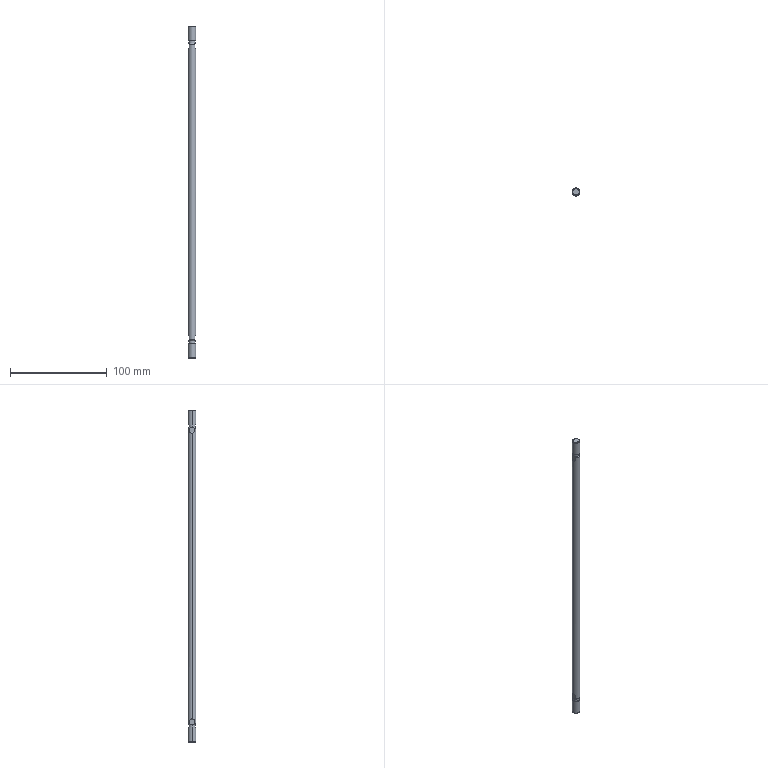Part | STEP file | rod_A_CDM2WB20_100_C76_0_ | 1 solid | 34 faces | box 8 x 8 x 344 mm | volume 17104 mm3 | plane 16 | cylinder 10 | cone 8 | commonest cylinder face diameters 8 x6 6.47 x4
STEP:
#1=CARTESIAN_POINT('',(3.235,0.,-316.));
#2=VERTEX_POINT('',#1);
#3=CARTESIAN_POINT('',(-3.235,0.,-316.));
#4=VERTEX_POINT('',#3);
#5=CARTESIAN_POINT('',(0.,0.,-316.));
#6=DIRECTION('',(0.,0.,1.));
#7=DIRECTION('',(1.,0.,0.));
#8=AXIS2_PLACEMENT_3D('',#5,#6,#7);
#9=CIRCLE('',#8,3.235);
#10=EDGE_CURVE('',#2,#4,#9,.T.);
#11=ORIENTED_EDGE('',*,*,#10,.T.);
#12=CARTESIAN_POINT('',(-4.,0.,-315.235));
#13=VERTEX_POINT('',#12);
#14=CARTESIAN_POINT('',(-3.235,0.,-316.));
#15=DIRECTION('',(-0.7071,0.,0.7071));
#16=VECTOR('',#15,1000.);
#17=LINE('',#14,#16);
#18=EDGE_CURVE('',#4,#13,#17,.T.);
#19=ORIENTED_EDGE('',*,*,#18,.T.);
#20=CARTESIAN_POINT('',(4.,0.,-315.235));
#21=VERTEX_POINT('',#20);
#22=CARTESIAN_POINT('',(0.,0.,-315.235));
#23=DIRECTION('',(0.,0.,1.));
#24=DIRECTION('',(1.,0.,0.));
#25=AXIS2_PLACEMENT_3D('',#22,#23,#24);
#26=CIRCLE('',#25,4.);
#27=EDGE_CURVE('',#21,#13,#26,.T.);
#28=ORIENTED_EDGE('',*,*,#27,.F.);
#29=CARTESIAN_POINT('',(3.235,0.,-316.));
#30=DIRECTION('',(0.7071,0.,0.7071));
#31=VECTOR('',#30,1000.);
#32=LINE('',#29,#31);
#33=EDGE_CURVE('',#2,#21,#32,.T.);
#34=ORIENTED_EDGE('',*,*,#33,.F.);
#35=EDGE_LOOP('',(#11,#19,#28,#34));
#36=FACE_OUTER_BOUND('',#35,.T.);
#37=CARTESIAN_POINT('',(0.,0.,-316.));
#38=DIRECTION('',(0.,0.,1.));
#39=DIRECTION('',(1.,0.,0.));
#40=AXIS2_PLACEMENT_3D('',#37,#38,#39);
#41=CONICAL_SURFACE('',#40,3.235,0.7854);
#42=ADVANCED_FACE('',(#36),#41,.T.);
#43=ORIENTED_EDGE('',*,*,#27,.T.);
#44=CARTESIAN_POINT('',(-4.,0.,-300.5));
#45=VERTEX_POINT('',#44);
#46=CARTESIAN_POINT('',(-4.,0.,-316.));
#47=DIRECTION('',(0.,0.,1.));
#48=VECTOR('',#47,1000.);
#49=LINE('',#46,#48);
#50=EDGE_CURVE('',#13,#45,#49,.T.);
#51=ORIENTED_EDGE('',*,*,#50,.T.);
#52=CARTESIAN_POINT('',(4.,0.,-300.5));
#53=VERTEX_POINT('',#52);
#54=CARTESIAN_POINT('',(0.,0.,-300.5));
#55=DIRECTION('',(0.,0.,1.));
#56=DIRECTION('',(1.,0.,0.));
#57=AXIS2_PLACEMENT_3D('',#54,#55,#56);
#58=CIRCLE('',#57,4.);
#59=EDGE_CURVE('',#53,#45,#58,.T.);
#60=ORIENTED_EDGE('',*,*,#59,.F.);
#61=CARTESIAN_POINT('',(4.,0.,-316.));
#62=DIRECTION('',(0.,0.,1.));
#63=VECTOR('',#62,1000.);
#64=LINE('',#61,#63);
#65=EDGE_CURVE('',#21,#53,#64,.T.);
#66=ORIENTED_EDGE('',*,*,#65,.F.);
#67=EDGE_LOOP('',(#43,#51,#60,#66));
#68=FACE_OUTER_BOUND('',#67,.T.);
#69=CARTESIAN_POINT('',(0.,0.,-316.));
#70=DIRECTION('',(0.,0.,1.));
#71=DIRECTION('',(1.,0.,0.));
#72=AXIS2_PLACEMENT_3D('',#69,#70,#71);
#73=CYLINDRICAL_SURFACE('',#72,4.);
#74=ADVANCED_FACE('',(#68),#73,.T.);
#75=CARTESIAN_POINT('',(3.235,0.,-300.5));
#76=VERTEX_POINT('',#75);
#77=CARTESIAN_POINT('',(-3.235,0.,-300.5));
#78=VERTEX_POINT('',#77);
#79=CARTESIAN_POINT('',(0.,0.,-300.5));
#80=DIRECTION('',(0.,0.,1.));
#81=DIRECTION('',(1.,0.,0.));
#82=AXIS2_PLACEMENT_3D('',#79,#80,#81);
#83=CIRCLE('',#82,3.235);
#84=EDGE_CURVE('',#76,#78,#83,.T.);
#85=ORIENTED_EDGE('',*,*,#84,.T.);
#86=CARTESIAN_POINT('',(-3.235,0.,-298.));
#87=VERTEX_POINT('',#86);
#88=CARTESIAN_POINT('',(-3.235,0.,-316.));
#89=DIRECTION('',(0.,0.,1.));
#90=VECTOR('',#89,1000.);
#91=LINE('',#88,#90);
#92=EDGE_CURVE('',#78,#87,#91,.T.);
#93=ORIENTED_EDGE('',*,*,#92,.T.);
#94=CARTESIAN_POINT('',(-3.,1.21,-298.));
#95=VERTEX_POINT('',#94);
#96=CARTESIAN_POINT('',(0.,0.,-298.));
#97=DIRECTION('',(0.,0.,1.));
#98=DIRECTION('',(1.,0.,0.));
#99=AXIS2_PLACEMENT_3D('',#96,#97,#98);
#100=CIRCLE('',#99,3.235);
#101=EDGE_CURVE('',#95,#87,#100,.T.);
#102=ORIENTED_EDGE('',*,*,#101,.F.);
#103=CARTESIAN_POINT('',(3.,1.21,-298.));
#104=VERTEX_POINT('',#103);
#105=CARTESIAN_POINT('',(0.,0.,-298.));
#106=DIRECTION('',(0.,0.,1.));
#107=DIRECTION('',(1.,0.,0.));
#108=AXIS2_PLACEMENT_3D('',#105,#106,#107);
#109=CIRCLE('',#108,3.235);
#110=EDGE_CURVE('',#104,#95,#109,.T.);
#111=ORIENTED_EDGE('',*,*,#110,.F.);
#112=CARTESIAN_POINT('',(3.235,0.,-298.));
#113=VERTEX_POINT('',#112);
#114=CARTESIAN_POINT('',(0.,0.,-298.));
#115=DIRECTION('',(0.,0.,1.));
#116=DIRECTION('',(1.,0.,0.));
#117=AXIS2_PLACEMENT_3D('',#114,#115,#116);
#118=CIRCLE('',#117,3.235);
#119=EDGE_CURVE('',#113,#104,#118,.T.);
#120=ORIENTED_EDGE('',*,*,#119,.F.);
#121=CARTESIAN_POINT('',(3.235,0.,-316.));
#122=DIRECTION('',(0.,0.,1.));
#123=VECTOR('',#122,1000.);
#124=LINE('',#121,#123);
#125=EDGE_CURVE('',#76,#113,#124,.T.);
#126=ORIENTED_EDGE('',*,*,#125,.F.);
#127=EDGE_LOOP('',(#85,#93,#102,#111,#120,#126));
#128=FACE_OUTER_BOUND('',#127,.T.);
#129=CARTESIAN_POINT('',(0.,0.,-316.));
#130=DIRECTION('',(0.,0.,1.));
#131=DIRECTION('',(1.,0.,0.));
#132=AXIS2_PLACEMENT_3D('',#129,#130,#131);
#133=CYLINDRICAL_SURFACE('',#132,3.235);
#134=ADVANCED_FACE('',(#128),#133,.T.);
#135=CARTESIAN_POINT('',(-3.,2.646,-293.));
#136=VERTEX_POINT('',#135);
#137=CARTESIAN_POINT('',(-4.,0.,-292.));
#138=VERTEX_POINT('',#137);
#139=CARTESIAN_POINT('',(-3.,2.646,-293.));
#140=CARTESIAN_POINT('',(-3.652,1.907,-292.348));
#141=CARTESIAN_POINT('',(-4.,0.9852,-292.));
#142=CARTESIAN_POINT('',(-4.,0.,-292.));
#143=(BOUNDED_CURVE()B_SPLINE_CURVE(3,(#139,#140,#141,#142),.UNSPECIFIED.,.F.,.F.)B_SPLINE_CURVE_WITH_KNOTS((4,4),(5.56,6.283),.UNSPECIFIED.)CURVE()GEOMETRIC_REPRESENTATION_ITEM()RATIONAL_B_SPLINE_CURVE((1.,0.9569,0.9569,1.))REPRESENTATION_ITEM(''));
#144=EDGE_CURVE('',#136,#138,#143,.T.);
#145=ORIENTED_EDGE('',*,*,#144,.T.);
#146=CARTESIAN_POINT('',(-4.,0.,4.));
#147=VERTEX_POINT('',#146);
#148=CARTESIAN_POINT('',(-4.,0.,-316.));
#149=DIRECTION('',(0.,0.,1.));
#150=VECTOR('',#149,1000.);
#151=LINE('',#148,#150);
#152=EDGE_CURVE('',#138,#147,#151,.T.);
#153=ORIENTED_EDGE('',*,*,#152,.T.);
#154=CARTESIAN_POINT('',(-3.,2.646,5.));
#155=VERTEX_POINT('',#154);
#156=CARTESIAN_POINT('',(-4.,0.,4.));
#157=CARTESIAN_POINT('',(-4.,0.9852,4.));
#158=CARTESIAN_POINT('',(-3.652,1.907,4.348));
#159=CARTESIAN_POINT('',(-3.,2.646,5.));
#160=(BOUNDED_CURVE()B_SPLINE_CURVE(3,(#156,#157,#158,#159),.UNSPECIFIED.,.F.,.F.)B_SPLINE_CURVE_WITH_KNOTS((4,4),(3.142,3.864),.UNSPECIFIED.)CURVE()GEOMETRIC_REPRESENTATION_ITEM()RATIONAL_B_SPLINE_CURVE((1.,0.9569,0.9569,1.))REPRESENTATION_ITEM(''));
#161=EDGE_CURVE('',#147,#155,#160,.T.);
#162=ORIENTED_EDGE('',*,*,#161,.T.);
#163=CARTESIAN_POINT('',(-3.,2.646,9.235));
#164=VERTEX_POINT('',#163);
#165=CARTESIAN_POINT('',(-3.,2.646,-316.));
#166=DIRECTION('',(0.,0.,1.));
#167=VECTOR('',#166,1000.);
#168=LINE('',#165,#167);
#169=EDGE_CURVE('',#155,#164,#168,.T.);
#170=ORIENTED_EDGE('',*,*,#169,.T.);
#171=CARTESIAN_POINT('',(3.,2.646,9.235));
#172=VERTEX_POINT('',#171);
#173=CARTESIAN_POINT('',(0.,0.,9.235));
#174=DIRECTION('',(0.,0.,1.));
#175=DIRECTION('',(1.,0.,0.));
#176=AXIS2_PLACEMENT_3D('',#173,#174,#175);
#177=CIRCLE('',#176,4.);
#178=EDGE_CURVE('',#172,#164,#177,.T.);
#179=ORIENTED_EDGE('',*,*,#178,.F.);
#180=CARTESIAN_POINT('',(3.,2.646,5.));
#181=VERTEX_POINT('',#180);
#182=CARTESIAN_POINT('',(3.,2.646,-316.));
#183=DIRECTION('',(0.,0.,-1.));
#184=VECTOR('',#183,1000.);
#185=LINE('',#182,#184);
#186=EDGE_CURVE('',#172,#181,#185,.T.);
#187=ORIENTED_EDGE('',*,*,#186,.T.);
#188=CARTESIAN_POINT('',(4.,0.,4.));
#189=VERTEX_POINT('',#188);
#190=CARTESIAN_POINT('',(3.,2.646,5.));
#191=CARTESIAN_POINT('',(3.652,1.907,4.348));
#192=CARTESIAN_POINT('',(4.,0.9852,4.));
#193=CARTESIAN_POINT('',(4.,0.,4.));
#194=(BOUNDED_CURVE()B_SPLINE_CURVE(3,(#190,#191,#192,#193),.UNSPECIFIED.,.F.,.F.)B_SPLINE_CURVE_WITH_KNOTS((4,4),(2.419,3.142),.UNSPECIFIED.)CURVE()GEOMETRIC_REPRESENTATION_ITEM()RATIONAL_B_SPLINE_CURVE((1.,0.9569,0.9569,1.))REPRESENTATION_ITEM(''));
#195=EDGE_CURVE('',#181,#189,#194,.T.);
#196=ORIENTED_EDGE('',*,*,#195,.T.);
#197=CARTESIAN_POINT('',(4.,0.,-292.));
#198=VERTEX_POINT('',#197);
#199=CARTESIAN_POINT('',(4.,0.,-316.));
#200=DIRECTION('',(0.,0.,1.));
#201=VECTOR('',#200,1000.);
#202=LINE('',#199,#201);
#203=EDGE_CURVE('',#198,#189,#202,.T.);
#204=ORIENTED_EDGE('',*,*,#203,.F.);
#205=CARTESIAN_POINT('',(3.,2.646,-293.));
#206=VERTEX_POINT('',#205);
#207=CARTESIAN_POINT('',(4.,0.,-292.));
#208=CARTESIAN_POINT('',(4.,0.9852,-292.));
#209=CARTESIAN_POINT('',(3.652,1.907,-292.348));
#210=CARTESIAN_POINT('',(3.,2.646,-293.));
#211=(BOUNDED_CURVE()B_SPLINE_CURVE(3,(#207,#208,#209,#210),.UNSPECIFIED.,.F.,.F.)B_SPLINE_CURVE_WITH_KNOTS((4,4),(0.,0.7227),.UNSPECIFIED.)CURVE()GEOMETRIC_REPRESENTATION_ITEM()RATIONAL_B_SPLINE_CURVE((1.,0.9569,0.9569,1.))REPRESENTATION_ITEM(''));
#212=EDGE_CURVE('',#198,#206,#211,.T.);
#213=ORIENTED_EDGE('',*,*,#212,.T.);
#214=CARTESIAN_POINT('',(3.,2.646,-297.235));
#215=VERTEX_POINT('',#214);
#216=CARTESIAN_POINT('',(3.,2.646,-316.));
#217=DIRECTION('',(0.,0.,-1.));
#218=VECTOR('',#217,1000.);
#219=LINE('',#216,#218);
#220=EDGE_CURVE('',#206,#215,#219,.T.);
#221=ORIENTED_EDGE('',*,*,#220,.T.);
#222=CARTESIAN_POINT('',(-3.,2.646,-297.235));
#223=VERTEX_POINT('',#222);
#224=CARTESIAN_POINT('',(0.,0.,-297.235));
#225=DIRECTION('',(0.,0.,1.));
#226=DIRECTION('',(1.,0.,0.));
#227=AXIS2_PLACEMENT_3D('',#224,#225,#226);
#228=CIRCLE('',#227,4.);
#229=EDGE_CURVE('',#215,#223,#228,.T.);
#230=ORIENTED_EDGE('',*,*,#229,.T.);
#231=CARTESIAN_POINT('',(-3.,2.646,-316.));
#232=DIRECTION('',(0.,0.,1.));
#233=VECTOR('',#232,1000.);
#234=LINE('',#231,#233);
#235=EDGE_CURVE('',#223,#136,#234,.T.);
#236=ORIENTED_EDGE('',*,*,#235,.T.);
#237=EDGE_LOOP('',(#145,#153,#162,#170,#179,#187,#196,#204,#213,#221,#230,#236));
#238=FACE_OUTER_BOUND('',#237,.T.);
#239=CARTESIAN_POINT('',(0.,0.,-316.));
#240=DIRECTION('',(0.,0.,1.));
#241=DIRECTION('',(1.,0.,0.));
#242=AXIS2_PLACEMENT_3D('',#239,#240,#241);
#243=CYLINDRICAL_SURFACE('',#242,4.);
#244=ADVANCED_FACE('',(#238),#243,.T.);
#245=CARTESIAN_POINT('',(-3.,1.21,10.));
#246=VERTEX_POINT('',#245);
#247=CARTESIAN_POINT('',(-3.235,0.,10.));
#248=VERTEX_POINT('',#247);
#249=CARTESIAN_POINT('',(0.,0.,10.));
#250=DIRECTION('',(0.,0.,1.));
#251=DIRECTION('',(1.,0.,0.));
#252=AXIS2_PLACEMENT_3D('',#249,#250,#251);
#253=CIRCLE('',#252,3.235);
#254=EDGE_CURVE('',#246,#248,#253,.T.);
#255=ORIENTED_EDGE('',*,*,#254,.T.);
#256=CARTESIAN_POINT('',(-3.235,0.,12.5));
#257=VERTEX_POINT('',#256);
#258=CARTESIAN_POINT('',(-3.235,0.,-316.));
#259=DIRECTION('',(0.,0.,1.));
#260=VECTOR('',#259,1000.);
#261=LINE('',#258,#260);
#262=EDGE_CURVE('',#248,#257,#261,.T.);
#263=ORIENTED_EDGE('',*,*,#262,.T.);
#264=CARTESIAN_POINT('',(3.235,0.,12.5));
#265=VERTEX_POINT('',#264);
#266=CARTESIAN_POINT('',(0.,0.,12.5));
#267=DIRECTION('',(0.,0.,1.));
#268=DIRECTION('',(1.,0.,0.));
#269=AXIS2_PLACEMENT_3D('',#266,#267,#268);
#270=CIRCLE('',#269,3.235);
#271=EDGE_CURVE('',#265,#257,#270,.T.);
#272=ORIENTED_EDGE('',*,*,#271,.F.);
#273=CARTESIAN_POINT('',(3.235,0.,10.));
#274=VERTEX_POINT('',#273);
#275=CARTESIAN_POINT('',(3.235,0.,-316.));
#276=DIRECTION('',(0.,0.,1.));
#277=VECTOR('',#276,1000.);
#278=LINE('',#275,#277);
#279=EDGE_CURVE('',#274,#265,#278,.T.);
#280=ORIENTED_EDGE('',*,*,#279,.F.);
#281=CARTESIAN_POINT('',(3.,1.21,10.));
#282=VERTEX_POINT('',#281);
#283=CARTESIAN_POINT('',(0.,0.,10.));
#284=DIRECTION('',(0.,0.,1.));
#285=DIRECTION('',(1.,0.,0.));
#286=AXIS2_PLACEMENT_3D('',#283,#284,#285);
#287=CIRCLE('',#286,3.235);
#288=EDGE_CURVE('',#274,#282,#287,.T.);
#289=ORIENTED_EDGE('',*,*,#288,.T.);
#290=CARTESIAN_POINT('',(0.,0.,10.));
#291=DIRECTION('',(0.,0.,1.));
#292=DIRECTION('',(1.,0.,0.));
#293=AXIS2_PLACEMENT_3D('',#290,#291,#292);
#294=CIRCLE('',#293,3.235);
#295=EDGE_CURVE('',#282,#246,#294,.T.);
#296=ORIENTED_EDGE('',*,*,#295,.T.);
#297=EDGE_LOOP('',(#255,#263,#272,#280,#289,#296));
#298=FACE_OUTER_BOUND('',#297,.T.);
#299=CARTESIAN_POINT('',(0.,0.,-316.));
#300=DIRECTION('',(0.,0.,1.));
#301=DIRECTION('',(1.,0.,0.));
#302=AXIS2_PLACEMENT_3D('',#299,#300,#301);
#303=CYLINDRICAL_SURFACE('',#302,3.235);
#304=ADVANCED_FACE('',(#298),#303,.T.);
#305=CARTESIAN_POINT('',(4.,0.,12.5));
#306=VERTEX_POINT('',#305);
#307=CARTESIAN_POINT('',(-4.,0.,12.5));
#308=VERTEX_POINT('',#307);
#309=CARTESIAN_POINT('',(0.,0.,12.5));
#310=DIRECTION('',(0.,0.,1.));
#311=DIRECTION('',(1.,0.,0.));
#312=AXIS2_PLACEMENT_3D('',#309,#310,#311);
#313=CIRCLE('',#312,4.);
#314=EDGE_CURVE('',#306,#308,#313,.T.);
#315=ORIENTED_EDGE('',*,*,#314,.T.);
#316=CARTESIAN_POINT('',(-4.,0.,27.235));
#317=VERTEX_POINT('',#316);
#318=CARTESIAN_POINT('',(-4.,0.,-316.));
#319=DIRECTION('',(0.,0.,1.));
#320=VECTOR('',#319,1000.);
#321=LINE('',#318,#320);
#322=EDGE_CURVE('',#308,#317,#321,.T.);
#323=ORIENTED_EDGE('',*,*,#322,.T.);
#324=CARTESIAN_POINT('',(4.,0.,27.235));
#325=VERTEX_POINT('',#324);
#326=CARTESIAN_POINT('',(0.,0.,27.235));
#327=DIRECTION('',(0.,0.,1.));
#328=DIRECTION('',(1.,0.,0.));
#329=AXIS2_PLACEMENT_3D('',#326,#327,#328);
#330=CIRCLE('',#329,4.);
#331=EDGE_CURVE('',#325,#317,#330,.T.);
#332=ORIENTED_EDGE('',*,*,#331,.F.);
#333=CARTESIAN_POINT('',(4.,0.,-316.));
#334=DIRECTION('',(0.,0.,1.));
#335=VECTOR('',#334,1000.);
#336=LINE('',#333,#335);
#337=EDGE_CURVE('',#306,#325,#336,.T.);
#338=ORIENTED_EDGE('',*,*,#337,.F.);
#339=EDGE_LOOP('',(#315,#323,#332,#338));
#340=FACE_OUTER_BOUND('',#339,.T.);
#341=CARTESIAN_POINT('',(0.,0.,-316.));
#342=DIRECTION('',(0.,0.,1.));
#343=DIRECTION('',(1.,0.,0.));
#344=AXIS2_PLACEMENT_3D('',#341,#342,#343);
#345=CYLINDRICAL_SURFACE('',#344,4.);
#346=ADVANCED_FACE('',(#340),#345,.T.);
#347=CARTESIAN_POINT('',(3.235,0.,28.));
#348=VERTEX_POINT('',#347);
#349=CARTESIAN_POINT('',(-3.235,0.,28.));
#350=VERTEX_POINT('',#349);
#351=CARTESIAN_POINT('',(0.,0.,28.));
#352=DIRECTION('',(0.,0.,1.));
#353=DIRECTION('',(1.,0.,0.));
#354=AXIS2_PLACEMENT_3D('',#351,#352,#353);
#355=CIRCLE('',#354,3.235);
#356=EDGE_CURVE('',#348,#350,#355,.T.);
#357=ORIENTED_EDGE('',*,*,#356,.F.);
#358=CARTESIAN_POINT('',(4.,0.,27.235));
#359=DIRECTION('',(0.7071,0.,-0.7071));
#360=VECTOR('',#359,1000.);
#361=LINE('',#358,#360);
#362=EDGE_CURVE('',#348,#325,#361,.T.);
#363=ORIENTED_EDGE('',*,*,#362,.T.);
#364=ORIENTED_EDGE('',*,*,#331,.T.);
#365=CARTESIAN_POINT('',(-4.,0.,27.235));
#366=DIRECTION('',(-0.7071,0.,-0.7071));
#367=VECTOR('',#366,1000.);
#368=LINE('',#365,#367);
#369=EDGE_CURVE('',#350,#317,#368,.T.);
#370=ORIENTED_EDGE('',*,*,#369,.F.);
#371=EDGE_LOOP('',(#357,#363,#364,#370));
#372=FACE_OUTER_BOUND('',#371,.T.);
#373=CARTESIAN_POINT('',(0.,0.,27.235));
#374=DIRECTION('',(0.,0.,-1.));
#375=DIRECTION('',(-1.,0.,0.));
#376=AXIS2_PLACEMENT_3D('',#373,#374,#375);
#377=CONICAL_SURFACE('',#376,4.,0.7854);
#378=ADVANCED_FACE('',(#372),#377,.T.);
#379=CARTESIAN_POINT('',(-3.,-2.646,-297.235));
#380=VERTEX_POINT('',#379);
#381=CARTESIAN_POINT('',(3.,-2.646,-297.235));
#382=VERTEX_POINT('',#381);
#383=CARTESIAN_POINT('',(0.,0.,-297.235));
#384=DIRECTION('',(0.,0.,1.));
#385=DIRECTION('',(1.,0.,0.));
#386=AXIS2_PLACEMENT_3D('',#383,#384,#385);
#387=CIRCLE('',#386,4.);
#388=EDGE_CURVE('',#380,#382,#387,.T.);
#389=ORIENTED_EDGE('',*,*,#388,.F.);
#390=CARTESIAN_POINT('',(-3.,-1.21,-298.));
#391=VERTEX_POINT('',#390);
#392=CARTESIAN_POINT('',(-3.,-2.646,-297.235));
#393=CARTESIAN_POINT('',(-3.,-2.421,-297.384));
#394=CARTESIAN_POINT('',(-3.,-2.191,-297.525));
#395=CARTESIAN_POINT('',(-3.,-1.715,-297.785));
#396=CARTESIAN_POINT('',(-3.,-1.466,-297.904));
#397=CARTESIAN_POINT('',(-3.,-1.21,-298.));
#398=B_SPLINE_CURVE_WITH_KNOTS('',3,(#392,#393,#394,#395,#396,#397),.UNSPECIFIED.,.F.,.F.,(4,2,4),(0.007443,0.008254,0.009065),.UNSPECIFIED.);
#399=EDGE_CURVE('',#380,#391,#398,.T.);
#400=ORIENTED_EDGE('',*,*,#399,.T.);
#401=CARTESIAN_POINT('',(3.,-1.21,-298.));
#402=VERTEX_POINT('',#401);
#403=CARTESIAN_POINT('',(0.,0.,-298.));
#404=DIRECTION('',(0.,0.,1.));
#405=DIRECTION('',(1.,0.,0.));
#406=AXIS2_PLACEMENT_3D('',#403,#404,#405);
#407=CIRCLE('',#406,3.235);
#408=EDGE_CURVE('',#391,#402,#407,.T.);
#409=ORIENTED_EDGE('',*,*,#408,.T.);
#410=CARTESIAN_POINT('',(3.,-1.21,-298.));
#411=CARTESIAN_POINT('',(3.,-1.465,-297.905));
#412=CARTESIAN_POINT('',(3.,-1.709,-297.788));
#413=CARTESIAN_POINT('',(3.,-2.186,-297.528));
#414=CARTESIAN_POINT('',(3.,-2.419,-297.385));
#415=CARTESIAN_POINT('',(3.,-2.646,-297.235));
#416=B_SPLINE_CURVE_WITH_KNOTS('',3,(#410,#411,#412,#413,#414,#415),.UNSPECIFIED.,.F.,.F.,(4,2,4),(0.01152,0.01233,0.01314),.UNSPECIFIED.);
#417=EDGE_CURVE('',#402,#382,#416,.T.);
#418=ORIENTED_EDGE('',*,*,#417,.T.);
#419=EDGE_LOOP('',(#389,#400,#409,#418));
#420=FACE_OUTER_BOUND('',#419,.T.);
#421=CARTESIAN_POINT('',(0.,0.,-298.));
#422=DIRECTION('',(0.,0.,1.));
#423=DIRECTION('',(1.,0.,0.));
#424=AXIS2_PLACEMENT_3D('',#421,#422,#423);
#425=CONICAL_SURFACE('',#424,3.235,0.7854);
#426=ADVANCED_FACE('',(#420),#425,.T.);
#427=ORIENTED_EDGE('',*,*,#178,.T.);
#428=CARTESIAN_POINT('',(-3.,2.646,9.235));
#429=CARTESIAN_POINT('',(-3.,2.421,9.384));
#430=CARTESIAN_POINT('',(-3.,2.191,9.525));
#431=CARTESIAN_POINT('',(-3.,1.715,9.785));
#432=CARTESIAN_POINT('',(-3.,1.466,9.904));
#433=CARTESIAN_POINT('',(-3.,1.21,10.));
#434=B_SPLINE_CURVE_WITH_KNOTS('',3,(#428,#429,#430,#431,#432,#433),.UNSPECIFIED.,.F.,.F.,(4,2,4),(0.007443,0.008254,0.009065),.UNSPECIFIED.);
#435=EDGE_CURVE('',#164,#246,#434,.T.);
#436=ORIENTED_EDGE('',*,*,#435,.T.);
#437=ORIENTED_EDGE('',*,*,#295,.F.);
#438=CARTESIAN_POINT('',(3.,1.21,10.));
#439=CARTESIAN_POINT('',(3.,1.465,9.905));
#440=CARTESIAN_POINT('',(3.,1.709,9.788));
#441=CARTESIAN_POINT('',(3.,2.186,9.528));
#442=CARTESIAN_POINT('',(3.,2.419,9.385));
#443=CARTESIAN_POINT('',(3.,2.646,9.235));
#444=B_SPLINE_CURVE_WITH_KNOTS('',3,(#438,#439,#440,#441,#442,#443),.UNSPECIFIED.,.F.,.F.,(4,2,4),(0.01152,0.01233,0.01314),.UNSPECIFIED.);
#445=EDGE_CURVE('',#282,#172,#444,.T.);
#446=ORIENTED_EDGE('',*,*,#445,.T.);
#447=EDGE_LOOP('',(#427,#436,#437,#446));
#448=FACE_OUTER_BOUND('',#447,.T.);
#449=CARTESIAN_POINT('',(0.,0.,9.235));
#450=DIRECTION('',(0.,0.,-1.));
#451=DIRECTION('',(-1.,0.,0.));
#452=AXIS2_PLACEMENT_3D('',#449,#450,#451);
#453=CONICAL_SURFACE('',#452,4.,0.7854);
#454=ADVANCED_FACE('',(#448),#453,.T.);
#455=CARTESIAN_POINT('',(0.,0.,28.));
#456=DIRECTION('',(0.,0.,1.));
#457=DIRECTION('',(1.,0.,0.));
#458=AXIS2_PLACEMENT_3D('',#455,#456,#457);
#459=CIRCLE('',#458,3.235);
#460=EDGE_CURVE('',#350,#348,#459,.T.);
#461=ORIENTED_EDGE('',*,*,#460,.T.);
#462=ORIENTED_EDGE('',*,*,#356,.T.);
#463=EDGE_LOOP('',(#461,#462));
#464=FACE_OUTER_BOUND('',#463,.T.);
#465=CARTESIAN_POINT('',(0.,0.,28.));
#466=DIRECTION('',(0.,0.,-1.));
#467=DIRECTION('',(-1.,0.,0.));
#468=AXIS2_PLACEMENT_3D('',#465,#466,#467);
#469=PLANE('',#468);
#470=ADVANCED_FACE('',(#464),#469,.F.);
#471=ORIENTED_EDGE('',*,*,#362,.F.);
#472=ORIENTED_EDGE('',*,*,#460,.F.);
#473=ORIENTED_EDGE('',*,*,#369,.T.);
#474=CARTESIAN_POINT('',(0.,0.,27.235));
#475=DIRECTION('',(0.,0.,1.));
#476=DIRECTION('',(1.,0.,0.));
#477=AXIS2_PLACEMENT_3D('',#474,#475,#476);
#478=CIRCLE('',#477,4.);
#479=EDGE_CURVE('',#317,#325,#478,.T.);
#480=ORIENTED_EDGE('',*,*,#479,.T.);
#481=EDGE_LOOP('',(#471,#472,#473,#480));
#482=FACE_OUTER_BOUND('',#481,.T.);
#483=CARTESIAN_POINT('',(0.,0.,27.235));
#484=DIRECTION('',(0.,0.,-1.));
#485=DIRECTION('',(-1.,0.,0.));
#486=AXIS2_PLACEMENT_3D('',#483,#484,#485);
#487=CONICAL_SURFACE('',#486,4.,0.7854);
#488=ADVANCED_FACE('',(#482),#487,.T.);
#489=ORIENTED_EDGE('',*,*,#322,.F.);
#490=CARTESIAN_POINT('',(0.,0.,12.5));
#491=DIRECTION('',(0.,0.,1.));
#492=DIRECTION('',(1.,0.,0.));
#493=AXIS2_PLACEMENT_3D('',#490,#491,#492);
#494=CIRCLE('',#493,4.);
#495=EDGE_CURVE('',#308,#306,#494,.T.);
#496=ORIENTED_EDGE('',*,*,#495,.T.);
#497=ORIENTED_EDGE('',*,*,#337,.T.);
#498=ORIENTED_EDGE('',*,*,#479,.F.);
#499=EDGE_LOOP('',(#489,#496,#497,#498));
#500=FACE_OUTER_BOUND('',#499,.T.);
#501=CARTESIAN_POINT('',(0.,0.,-316.));
#502=DIRECTION('',(0.,0.,1.));
#503=DIRECTION('',(1.,0.,0.));
#504=AXIS2_PLACEMENT_3D('',#501,#502,#503);
#505=CYLINDRICAL_SURFACE('',#504,4.);
#506=ADVANCED_FACE('',(#500),#505,.T.);
#507=ORIENTED_EDGE('',*,*,#314,.F.);
#508=ORIENTED_EDGE('',*,*,#495,.F.);
#509=EDGE_LOOP('',(#507,#508));
#510=FACE_OUTER_BOUND('',#509,.T.);
#511=ORIENTED_EDGE('',*,*,#271,.T.);
#512=CARTESIAN_POINT('',(0.,0.,12.5));
#513=DIRECTION('',(0.,0.,1.));
#514=DIRECTION('',(1.,0.,0.));
#515=AXIS2_PLACEMENT_3D('',#512,#513,#514);
#516=CIRCLE('',#515,3.235);
#517=EDGE_CURVE('',#257,#265,#516,.T.);
#518=ORIENTED_EDGE('',*,*,#517,.T.);
#519=EDGE_LOOP('',(#511,#518));
#520=FACE_BOUND('',#519,.T.);
#521=CARTESIAN_POINT('',(0.,4.,12.5));
#522=DIRECTION('',(0.,0.,1.));
#523=DIRECTION('',(1.,0.,0.));
#524=AXIS2_PLACEMENT_3D('',#521,#522,#523);
#525=PLANE('',#524);
#526=ADVANCED_FACE('',(#510,#520),#525,.F.);
#527=ORIENTED_EDGE('',*,*,#262,.F.);
#528=CARTESIAN_POINT('',(-3.,-1.21,10.));
#529=VERTEX_POINT('',#528);
#530=CARTESIAN_POINT('',(0.,0.,10.));
#531=DIRECTION('',(0.,0.,1.));
#532=DIRECTION('',(1.,0.,0.));
#533=AXIS2_PLACEMENT_3D('',#530,#531,#532);
#534=CIRCLE('',#533,3.235);
#535=EDGE_CURVE('',#248,#529,#534,.T.);
#536=ORIENTED_EDGE('',*,*,#535,.T.);
#537=CARTESIAN_POINT('',(3.,-1.21,10.));
#538=VERTEX_POINT('',#537);
#539=CARTESIAN_POINT('',(0.,0.,10.));
#540=DIRECTION('',(0.,0.,1.));
#541=DIRECTION('',(1.,0.,0.));
#542=AXIS2_PLACEMENT_3D('',#539,#540,#541);
#543=CIRCLE('',#542,3.235);
#544=EDGE_CURVE('',#529,#538,#543,.T.);
#545=ORIENTED_EDGE('',*,*,#544,.T.);
#546=CARTESIAN_POINT('',(0.,0.,10.));
#547=DIRECTION('',(0.,0.,1.));
#548=DIRECTION('',(1.,0.,0.));
#549=AXIS2_PLACEMENT_3D('',#546,#547,#548);
#550=CIRCLE('',#549,3.235);
#551=EDGE_CURVE('',#538,#274,#550,.T.);
#552=ORIENTED_EDGE('',*,*,#551,.T.);
#553=ORIENTED_EDGE('',*,*,#279,.T.);
#554=ORIENTED_EDGE('',*,*,#517,.F.);
#555=EDGE_LOOP('',(#527,#536,#545,#552,#553,#554));
#556=FACE_OUTER_BOUND('',#555,.T.);
#557=CARTESIAN_POINT('',(0.,0.,-316.));
#558=DIRECTION('',(0.,0.,1.));
#559=DIRECTION('',(1.,0.,0.));
#560=AXIS2_PLACEMENT_3D('',#557,#558,#559);
#561=CYLINDRICAL_SURFACE('',#560,3.235);
#562=ADVANCED_FACE('',(#556),#561,.T.);
#563=ORIENTED_EDGE('',*,*,#544,.F.);
#564=CARTESIAN_POINT('',(-3.,-2.646,9.235));
#565=VERTEX_POINT('',#564);
#566=CARTESIAN_POINT('',(-3.,-1.21,10.));
#567=CARTESIAN_POINT('',(-3.,-1.465,9.905));
#568=CARTESIAN_POINT('',(-3.,-1.709,9.788));
#569=CARTESIAN_POINT('',(-3.,-2.186,9.528));
#570=CARTESIAN_POINT('',(-3.,-2.419,9.385));
#571=CARTESIAN_POINT('',(-3.,-2.646,9.235));
#572=B_SPLINE_CURVE_WITH_KNOTS('',3,(#566,#567,#568,#569,#570,#571),.UNSPECIFIED.,.F.,.F.,(4,2,4),(0.01152,0.01233,0.01314),.UNSPECIFIED.);
#573=EDGE_CURVE('',#529,#565,#572,.T.);
#574=ORIENTED_EDGE('',*,*,#573,.T.);
#575=CARTESIAN_POINT('',(3.,-2.646,9.235));
#576=VERTEX_POINT('',#575);
#577=CARTESIAN_POINT('',(0.,0.,9.235));
#578=DIRECTION('',(0.,0.,1.));
#579=DIRECTION('',(1.,0.,0.));
#580=AXIS2_PLACEMENT_3D('',#577,#578,#579);
#581=CIRCLE('',#580,4.);
#582=EDGE_CURVE('',#565,#576,#581,.T.);
#583=ORIENTED_EDGE('',*,*,#582,.T.);
#584=CARTESIAN_POINT('',(3.,-2.646,9.235));
#585=CARTESIAN_POINT('',(3.,-2.421,9.384));
#586=CARTESIAN_POINT('',(3.,-2.191,9.525));
#587=CARTESIAN_POINT('',(3.,-1.715,9.785));
#588=CARTESIAN_POINT('',(3.,-1.466,9.904));
#589=CARTESIAN_POINT('',(3.,-1.21,10.));
#590=B_SPLINE_CURVE_WITH_KNOTS('',3,(#584,#585,#586,#587,#588,#589),.UNSPECIFIED.,.F.,.F.,(4,2,4),(0.007443,0.008254,0.009065),.UNSPECIFIED.);
#591=EDGE_CURVE('',#576,#538,#590,.T.);
#592=ORIENTED_EDGE('',*,*,#591,.T.);
#593=EDGE_LOOP('',(#563,#574,#583,#592));
#594=FACE_OUTER_BOUND('',#593,.T.);
#595=CARTESIAN_POINT('',(0.,0.,9.235));
#596=DIRECTION('',(0.,0.,-1.));
#597=DIRECTION('',(-1.,0.,0.));
#598=AXIS2_PLACEMENT_3D('',#595,#596,#597);
#599=CONICAL_SURFACE('',#598,4.,0.7854);
#600=ADVANCED_FACE('',(#594),#599,.T.);
#601=ORIENTED_EDGE('',*,*,#152,.F.);
#602=CARTESIAN_POINT('',(-3.,-2.646,-293.));
#603=VERTEX_POINT('',#602);
#604=CARTESIAN_POINT('',(-4.,0.,-292.));
#605=CARTESIAN_POINT('',(-4.,-0.9852,-292.));
#606=CARTESIAN_POINT('',(-3.652,-1.907,-292.348));
#607=CARTESIAN_POINT('',(-3.,-2.646,-293.));
#608=(BOUNDED_CURVE()B_SPLINE_CURVE(3,(#604,#605,#606,#607),.UNSPECIFIED.,.F.,.F.)B_SPLINE_CURVE_WITH_KNOTS((4,4),(0.,0.7227),.UNSPECIFIED.)CURVE()GEOMETRIC_REPRESENTATION_ITEM()RATIONAL_B_SPLINE_CURVE((1.,0.9569,0.9569,1.))REPRESENTATION_ITEM(''));
#609=EDGE_CURVE('',#138,#603,#608,.T.);
#610=ORIENTED_EDGE('',*,*,#609,.T.);
#611=CARTESIAN_POINT('',(-3.,-2.646,-316.));
#612=DIRECTION('',(0.,0.,-1.));
#613=VECTOR('',#612,1000.);
#614=LINE('',#611,#613);
#615=EDGE_CURVE('',#603,#380,#614,.T.);
#616=ORIENTED_EDGE('',*,*,#615,.T.);
#617=ORIENTED_EDGE('',*,*,#388,.T.);
#618=CARTESIAN_POINT('',(3.,-2.646,-293.));
#619=VERTEX_POINT('',#618);
#620=CARTESIAN_POINT('',(3.,-2.646,-316.));
#621=DIRECTION('',(0.,0.,1.));
#622=VECTOR('',#621,1000.);
#623=LINE('',#620,#622);
#624=EDGE_CURVE('',#382,#619,#623,.T.);
#625=ORIENTED_EDGE('',*,*,#624,.T.);
#626=CARTESIAN_POINT('',(3.,-2.646,-293.));
#627=CARTESIAN_POINT('',(3.652,-1.907,-292.348));
#628=CARTESIAN_POINT('',(4.,-0.9852,-292.));
#629=CARTESIAN_POINT('',(4.,0.,-292.));
#630=(BOUNDED_CURVE()B_SPLINE_CURVE(3,(#626,#627,#628,#629),.UNSPECIFIED.,.F.,.F.)B_SPLINE_CURVE_WITH_KNOTS((4,4),(5.56,6.283),.UNSPECIFIED.)CURVE()GEOMETRIC_REPRESENTATION_ITEM()RATIONAL_B_SPLINE_CURVE((1.,0.9569,0.9569,1.))REPRESENTATION_ITEM(''));
#631=EDGE_CURVE('',#619,#198,#630,.T.);
#632=ORIENTED_EDGE('',*,*,#631,.T.);
#633=ORIENTED_EDGE('',*,*,#203,.T.);
#634=CARTESIAN_POINT('',(3.,-2.646,5.));
#635=VERTEX_POINT('',#634);
#636=CARTESIAN_POINT('',(4.,0.,4.));
#637=CARTESIAN_POINT('',(4.,-0.9852,4.));
#638=CARTESIAN_POINT('',(3.652,-1.907,4.348));
#639=CARTESIAN_POINT('',(3.,-2.646,5.));
#640=(BOUNDED_CURVE()B_SPLINE_CURVE(3,(#636,#637,#638,#639),.UNSPECIFIED.,.F.,.T.)B_SPLINE_CURVE_WITH_KNOTS((4,4),(3.142,3.864),.UNSPECIFIED.)CURVE()GEOMETRIC_REPRESENTATION_ITEM()RATIONAL_B_SPLINE_CURVE((1.,0.9569,0.9569,1.))REPRESENTATION_ITEM(''));
#641=EDGE_CURVE('',#189,#635,#640,.T.);
#642=ORIENTED_EDGE('',*,*,#641,.T.);
#643=CARTESIAN_POINT('',(3.,-2.646,-316.));
#644=DIRECTION('',(0.,0.,1.));
#645=VECTOR('',#644,1000.);
#646=LINE('',#643,#645);
#647=EDGE_CURVE('',#635,#576,#646,.T.);
#648=ORIENTED_EDGE('',*,*,#647,.T.);
#649=ORIENTED_EDGE('',*,*,#582,.F.);
#650=CARTESIAN_POINT('',(-3.,-2.646,5.));
#651=VERTEX_POINT('',#650);
#652=CARTESIAN_POINT('',(-3.,-2.646,-316.));
#653=DIRECTION('',(0.,0.,-1.));
#654=VECTOR('',#653,1000.);
#655=LINE('',#652,#654);
#656=EDGE_CURVE('',#565,#651,#655,.T.);
#657=ORIENTED_EDGE('',*,*,#656,.T.);
#658=CARTESIAN_POINT('',(-3.,-2.646,5.));
#659=CARTESIAN_POINT('',(-3.652,-1.907,4.348));
#660=CARTESIAN_POINT('',(-4.,-0.9852,4.));
#661=CARTESIAN_POINT('',(-4.,0.,4.));
#662=(BOUNDED_CURVE()B_SPLINE_CURVE(3,(#658,#659,#660,#661),.UNSPECIFIED.,.F.,.F.)B_SPLINE_CURVE_WITH_KNOTS((4,4),(2.419,3.142),.UNSPECIFIED.)CURVE()GEOMETRIC_REPRESENTATION_ITEM()RATIONAL_B_SPLINE_CURVE((1.,0.9569,0.9569,1.))REPRESENTATION_ITEM(''));
#663=EDGE_CURVE('',#651,#147,#662,.T.);
#664=ORIENTED_EDGE('',*,*,#663,.T.);
#665=EDGE_LOOP('',(#601,#610,#616,#617,#625,#632,#633,#642,#648,#649,#657,#664));
#666=FACE_OUTER_BOUND('',#665,.T.);
#667=CARTESIAN_POINT('',(0.,0.,-316.));
#668=DIRECTION('',(0.,0.,1.));
#669=DIRECTION('',(1.,0.,0.));
#670=AXIS2_PLACEMENT_3D('',#667,#668,#669);
#671=CYLINDRICAL_SURFACE('',#670,4.);
#672=ADVANCED_FACE('',(#666),#671,.T.);
#673=ORIENTED_EDGE('',*,*,#110,.T.);
#674=CARTESIAN_POINT('',(-3.,1.21,-298.));
#675=CARTESIAN_POINT('',(-3.,1.465,-297.905));
#676=CARTESIAN_POINT('',(-3.,1.709,-297.788));
#677=CARTESIAN_POINT('',(-3.,2.186,-297.528));
#678=CARTESIAN_POINT('',(-3.,2.419,-297.385));
#679=CARTESIAN_POINT('',(-3.,2.646,-297.235));
#680=B_SPLINE_CURVE_WITH_KNOTS('',3,(#674,#675,#676,#677,#678,#679),.UNSPECIFIED.,.F.,.F.,(4,2,4),(0.01152,0.01233,0.01314),.UNSPECIFIED.);
#681=EDGE_CURVE('',#95,#223,#680,.T.);
#682=ORIENTED_EDGE('',*,*,#681,.T.);
#683=ORIENTED_EDGE('',*,*,#229,.F.);
#684=CARTESIAN_POINT('',(3.,2.646,-297.235));
#685=CARTESIAN_POINT('',(3.,2.421,-297.384));
#686=CARTESIAN_POINT('',(3.,2.191,-297.525));
#687=CARTESIAN_POINT('',(3.,1.715,-297.785));
#688=CARTESIAN_POINT('',(3.,1.466,-297.904));
#689=CARTESIAN_POINT('',(3.,1.21,-298.));
#690=B_SPLINE_CURVE_WITH_KNOTS('',3,(#684,#685,#686,#687,#688,#689),.UNSPECIFIED.,.F.,.F.,(4,2,4),(0.007443,0.008254,0.009065),.UNSPECIFIED.);
#691=EDGE_CURVE('',#215,#104,#690,.T.);
#692=ORIENTED_EDGE('',*,*,#691,.T.);
#693=EDGE_LOOP('',(#673,#682,#683,#692));
#694=FACE_OUTER_BOUND('',#693,.T.);
#695=CARTESIAN_POINT('',(0.,0.,-298.));
#696=DIRECTION('',(0.,0.,1.));
#697=DIRECTION('',(1.,0.,0.));
#698=AXIS2_PLACEMENT_3D('',#695,#696,#697);
#699=CONICAL_SURFACE('',#698,3.235,0.7854);
#700=ADVANCED_FACE('',(#694),#699,.T.);
#701=ORIENTED_EDGE('',*,*,#92,.F.);
#702=CARTESIAN_POINT('',(0.,0.,-300.5));
#703=DIRECTION('',(0.,0.,1.));
#704=DIRECTION('',(1.,0.,0.));
#705=AXIS2_PLACEMENT_3D('',#702,#703,#704);
#706=CIRCLE('',#705,3.235);
#707=EDGE_CURVE('',#78,#76,#706,.T.);
#708=ORIENTED_EDGE('',*,*,#707,.T.);
#709=ORIENTED_EDGE('',*,*,#125,.T.);
#710=CARTESIAN_POINT('',(0.,0.,-298.));
#711=DIRECTION('',(0.,0.,1.));
#712=DIRECTION('',(1.,0.,0.));
#713=AXIS2_PLACEMENT_3D('',#710,#711,#712);
#714=CIRCLE('',#713,3.235);
#715=EDGE_CURVE('',#402,#113,#714,.T.);
#716=ORIENTED_EDGE('',*,*,#715,.F.);
#717=ORIENTED_EDGE('',*,*,#408,.F.);
#718=CARTESIAN_POINT('',(0.,0.,-298.));
#719=DIRECTION('',(0.,0.,1.));
#720=DIRECTION('',(1.,0.,0.));
#721=AXIS2_PLACEMENT_3D('',#718,#719,#720);
#722=CIRCLE('',#721,3.235);
#723=EDGE_CURVE('',#87,#391,#722,.T.);
#724=ORIENTED_EDGE('',*,*,#723,.F.);
#725=EDGE_LOOP('',(#701,#708,#709,#716,#717,#724));
#726=FACE_OUTER_BOUND('',#725,.T.);
#727=CARTESIAN_POINT('',(0.,0.,-316.));
#728=DIRECTION('',(0.,0.,1.));
#729=DIRECTION('',(1.,0.,0.));
#730=AXIS2_PLACEMENT_3D('',#727,#728,#729);
#731=CYLINDRICAL_SURFACE('',#730,3.235);
#732=ADVANCED_FACE('',(#726),#731,.T.);
#733=ORIENTED_EDGE('',*,*,#84,.F.);
#734=ORIENTED_EDGE('',*,*,#707,.F.);
#735=EDGE_LOOP('',(#733,#734));
#736=FACE_BOUND('',#735,.T.);
#737=ORIENTED_EDGE('',*,*,#59,.T.);
#738=CARTESIAN_POINT('',(0.,0.,-300.5));
#739=DIRECTION('',(0.,0.,1.));
#740=DIRECTION('',(1.,0.,0.));
#741=AXIS2_PLACEMENT_3D('',#738,#739,#740);
#742=CIRCLE('',#741,4.);
#743=EDGE_CURVE('',#45,#53,#742,.T.);
#744=ORIENTED_EDGE('',*,*,#743,.T.);
#745=EDGE_LOOP('',(#737,#744));
#746=FACE_OUTER_BOUND('',#745,.T.);
#747=CARTESIAN_POINT('',(0.,3.235,-300.5));
#748=DIRECTION('',(0.,0.,-1.));
#749=DIRECTION('',(-1.,0.,0.));
#750=AXIS2_PLACEMENT_3D('',#747,#748,#749);
#751=PLANE('',#750);
#752=ADVANCED_FACE('',(#736,#746),#751,.F.);
#753=ORIENTED_EDGE('',*,*,#50,.F.);
#754=CARTESIAN_POINT('',(0.,0.,-315.235));
#755=DIRECTION('',(0.,0.,1.));
#756=DIRECTION('',(1.,0.,0.));
#757=AXIS2_PLACEMENT_3D('',#754,#755,#756);
#758=CIRCLE('',#757,4.);
#759=EDGE_CURVE('',#13,#21,#758,.T.);
#760=ORIENTED_EDGE('',*,*,#759,.T.);
#761=ORIENTED_EDGE('',*,*,#65,.T.);
#762=ORIENTED_EDGE('',*,*,#743,.F.);
#763=EDGE_LOOP('',(#753,#760,#761,#762));
#764=FACE_OUTER_BOUND('',#763,.T.);
#765=CARTESIAN_POINT('',(0.,0.,-316.));
#766=DIRECTION('',(0.,0.,1.));
#767=DIRECTION('',(1.,0.,0.));
#768=AXIS2_PLACEMENT_3D('',#765,#766,#767);
#769=CYLINDRICAL_SURFACE('',#768,4.);
#770=ADVANCED_FACE('',(#764),#769,.T.);
#771=ORIENTED_EDGE('',*,*,#18,.F.);
#772=CARTESIAN_POINT('',(0.,0.,-316.));
#773=DIRECTION('',(0.,0.,1.));
#774=DIRECTION('',(1.,0.,0.));
#775=AXIS2_PLACEMENT_3D('',#772,#773,#774);
#776=CIRCLE('',#775,3.235);
#777=EDGE_CURVE('',#4,#2,#776,.T.);
#778=ORIENTED_EDGE('',*,*,#777,.T.);
#779=ORIENTED_EDGE('',*,*,#33,.T.);
#780=ORIENTED_EDGE('',*,*,#759,.F.);
#781=EDGE_LOOP('',(#771,#778,#779,#780));
#782=FACE_OUTER_BOUND('',#781,.T.);
#783=CARTESIAN_POINT('',(0.,0.,-316.));
#784=DIRECTION('',(0.,0.,1.));
#785=DIRECTION('',(1.,0.,0.));
#786=AXIS2_PLACEMENT_3D('',#783,#784,#785);
#787=CONICAL_SURFACE('',#786,3.235,0.7854);
#788=ADVANCED_FACE('',(#782),#787,.T.);
#789=ORIENTED_EDGE('',*,*,#10,.F.);
#790=ORIENTED_EDGE('',*,*,#777,.F.);
#791=EDGE_LOOP('',(#789,#790));
#792=FACE_OUTER_BOUND('',#791,.T.);
#793=CARTESIAN_POINT('',(0.,3.235,-316.));
#794=DIRECTION('',(0.,0.,1.));
#795=DIRECTION('',(1.,0.,0.));
#796=AXIS2_PLACEMENT_3D('',#793,#794,#795);
#797=PLANE('',#796);
#798=ADVANCED_FACE('',(#792),#797,.F.);
#799=CARTESIAN_POINT('',(3.,-8.,10.));
#800=DIRECTION('',(0.,1.,0.));
#801=VECTOR('',#800,1000.);
#802=LINE('',#799,#801);
#803=EDGE_CURVE('',#538,#282,#802,.T.);
#804=ORIENTED_EDGE('',*,*,#803,.T.);
#805=ORIENTED_EDGE('',*,*,#288,.F.);
#806=ORIENTED_EDGE('',*,*,#551,.F.);
#807=EDGE_LOOP('',(#804,#805,#806));
#808=FACE_OUTER_BOUND('',#807,.T.);
#809=CARTESIAN_POINT('',(3.,-8.,10.));
#810=DIRECTION('',(0.,0.,1.));
#811=DIRECTION('',(1.,0.,0.));
#812=AXIS2_PLACEMENT_3D('',#809,#810,#811);
#813=PLANE('',#812);
#814=ADVANCED_FACE('',(#808),#813,.F.);
#815=ORIENTED_EDGE('',*,*,#647,.F.);
#816=CARTESIAN_POINT('',(3.,-8.,5.));
#817=DIRECTION('',(0.,1.,0.));
#818=VECTOR('',#817,1000.);
#819=LINE('',#816,#818);
#820=EDGE_CURVE('',#635,#181,#819,.T.);
#821=ORIENTED_EDGE('',*,*,#820,.T.);
#822=ORIENTED_EDGE('',*,*,#186,.F.);
#823=ORIENTED_EDGE('',*,*,#445,.F.);
#824=ORIENTED_EDGE('',*,*,#803,.F.);
#825=ORIENTED_EDGE('',*,*,#591,.F.);
#826=EDGE_LOOP('',(#815,#821,#822,#823,#824,#825));
#827=FACE_OUTER_BOUND('',#826,.T.);
#828=CARTESIAN_POINT('',(3.,-8.,5.));
#829=DIRECTION('',(-1.,0.,0.));
#830=DIRECTION('',(0.,0.,1.));
#831=AXIS2_PLACEMENT_3D('',#828,#829,#830);
#832=PLANE('',#831);
#833=ADVANCED_FACE('',(#827),#832,.F.);
#834=ORIENTED_EDGE('',*,*,#820,.F.);
#835=ORIENTED_EDGE('',*,*,#641,.F.);
#836=ORIENTED_EDGE('',*,*,#195,.F.);
#837=EDGE_LOOP('',(#834,#835,#836));
#838=FACE_OUTER_BOUND('',#837,.T.);
#839=CARTESIAN_POINT('',(4.,-8.,4.));
#840=DIRECTION('',(-0.7071,0.,-0.7071));
#841=DIRECTION('',(-0.7071,0.,0.7071));
#842=AXIS2_PLACEMENT_3D('',#839,#840,#841);
#843=PLANE('',#842);
#844=ADVANCED_FACE('',(#838),#843,.F.);
#845=CARTESIAN_POINT('',(-3.,-8.,10.));
#846=DIRECTION('',(0.,1.,0.));
#847=VECTOR('',#846,1000.);
#848=LINE('',#845,#847);
#849=EDGE_CURVE('',#529,#246,#848,.T.);
#850=ORIENTED_EDGE('',*,*,#849,.F.);
#851=ORIENTED_EDGE('',*,*,#535,.F.);
#852=ORIENTED_EDGE('',*,*,#254,.F.);
#853=EDGE_LOOP('',(#850,#851,#852));
#854=FACE_OUTER_BOUND('',#853,.T.);
#855=CARTESIAN_POINT('',(-6.,-8.,10.));
#856=DIRECTION('',(0.,0.,1.));
#857=DIRECTION('',(1.,0.,0.));
#858=AXIS2_PLACEMENT_3D('',#855,#856,#857);
#859=PLANE('',#858);
#860=ADVANCED_FACE('',(#854),#859,.F.);
#861=CARTESIAN_POINT('',(-3.,-8.,5.));
#862=DIRECTION('',(0.,1.,0.));
#863=VECTOR('',#862,1000.);
#864=LINE('',#861,#863);
#865=EDGE_CURVE('',#651,#155,#864,.T.);
#866=ORIENTED_EDGE('',*,*,#865,.T.);
#867=ORIENTED_EDGE('',*,*,#161,.F.);
#868=ORIENTED_EDGE('',*,*,#663,.F.);
#869=EDGE_LOOP('',(#866,#867,#868));
#870=FACE_OUTER_BOUND('',#869,.T.);
#871=CARTESIAN_POINT('',(-3.,-8.,5.));
#872=DIRECTION('',(0.7071,0.,-0.7071));
#873=DIRECTION('',(-0.7071,0.,-0.7071));
#874=AXIS2_PLACEMENT_3D('',#871,#872,#873);
#875=PLANE('',#874);
#876=ADVANCED_FACE('',(#870),#875,.F.);
#877=ORIENTED_EDGE('',*,*,#169,.F.);
#878=ORIENTED_EDGE('',*,*,#865,.F.);
#879=ORIENTED_EDGE('',*,*,#656,.F.);
#880=ORIENTED_EDGE('',*,*,#573,.F.);
#881=ORIENTED_EDGE('',*,*,#849,.T.);
#882=ORIENTED_EDGE('',*,*,#435,.F.);
#883=EDGE_LOOP('',(#877,#878,#879,#880,#881,#882));
#884=FACE_OUTER_BOUND('',#883,.T.);
#885=CARTESIAN_POINT('',(-3.,-8.,10.));
#886=DIRECTION('',(1.,0.,0.));
#887=DIRECTION('',(0.,0.,-1.));
#888=AXIS2_PLACEMENT_3D('',#885,#886,#887);
#889=PLANE('',#888);
#890=ADVANCED_FACE('',(#884),#889,.F.);
#891=ORIENTED_EDGE('',*,*,#631,.F.);
#892=CARTESIAN_POINT('',(3.,-8.,-293.));
#893=DIRECTION('',(0.,1.,0.));
#894=VECTOR('',#893,1000.);
#895=LINE('',#892,#894);
#896=EDGE_CURVE('',#619,#206,#895,.T.);
#897=ORIENTED_EDGE('',*,*,#896,.T.);
#898=ORIENTED_EDGE('',*,*,#212,.F.);
#899=EDGE_LOOP('',(#891,#897,#898));
#900=FACE_OUTER_BOUND('',#899,.T.);
#901=CARTESIAN_POINT('',(3.,-8.,-293.));
#902=DIRECTION('',(-0.7071,0.,0.7071));
#903=DIRECTION('',(0.7071,0.,0.7071));
#904=AXIS2_PLACEMENT_3D('',#901,#902,#903);
#905=PLANE('',#904);
#906=ADVANCED_FACE('',(#900),#905,.F.);
#907=ORIENTED_EDGE('',*,*,#896,.F.);
#908=ORIENTED_EDGE('',*,*,#624,.F.);
#909=ORIENTED_EDGE('',*,*,#417,.F.);
#910=CARTESIAN_POINT('',(3.,-8.,-298.));
#911=DIRECTION('',(0.,1.,0.));
#912=VECTOR('',#911,1000.);
#913=LINE('',#910,#912);
#914=EDGE_CURVE('',#402,#104,#913,.T.);
#915=ORIENTED_EDGE('',*,*,#914,.T.);
#916=ORIENTED_EDGE('',*,*,#691,.F.);
#917=ORIENTED_EDGE('',*,*,#220,.F.);
#918=EDGE_LOOP('',(#907,#908,#909,#915,#916,#917));
#919=FACE_OUTER_BOUND('',#918,.T.);
#920=CARTESIAN_POINT('',(3.,-8.,-298.));
#921=DIRECTION('',(-1.,0.,0.));
#922=DIRECTION('',(0.,0.,1.));
#923=AXIS2_PLACEMENT_3D('',#920,#921,#922);
#924=PLANE('',#923);
#925=ADVANCED_FACE('',(#919),#924,.F.);
#926=ORIENTED_EDGE('',*,*,#914,.F.);
#927=ORIENTED_EDGE('',*,*,#715,.T.);
#928=ORIENTED_EDGE('',*,*,#119,.T.);
#929=EDGE_LOOP('',(#926,#927,#928));
#930=FACE_OUTER_BOUND('',#929,.T.);
#931=CARTESIAN_POINT('',(6.,-8.,-298.));
#932=DIRECTION('',(0.,0.,-1.));
#933=DIRECTION('',(-1.,0.,0.));
#934=AXIS2_PLACEMENT_3D('',#931,#932,#933);
#935=PLANE('',#934);
#936=ADVANCED_FACE('',(#930),#935,.F.);
#937=ORIENTED_EDGE('',*,*,#144,.F.);
#938=CARTESIAN_POINT('',(-3.,-8.,-293.));
#939=DIRECTION('',(0.,1.,0.));
#940=VECTOR('',#939,1000.);
#941=LINE('',#938,#940);
#942=EDGE_CURVE('',#603,#136,#941,.T.);
#943=ORIENTED_EDGE('',*,*,#942,.F.);
#944=ORIENTED_EDGE('',*,*,#609,.F.);
#945=EDGE_LOOP('',(#937,#943,#944));
#946=FACE_OUTER_BOUND('',#945,.T.);
#947=CARTESIAN_POINT('',(-4.,-8.,-292.));
#948=DIRECTION('',(0.7071,0.,0.7071));
#949=DIRECTION('',(0.7071,0.,-0.7071));
#950=AXIS2_PLACEMENT_3D('',#947,#948,#949);
#951=PLANE('',#950);
#952=ADVANCED_FACE('',(#946),#951,.F.);
#953=ORIENTED_EDGE('',*,*,#942,.T.);
#954=ORIENTED_EDGE('',*,*,#235,.F.);
#955=ORIENTED_EDGE('',*,*,#681,.F.);
#956=CARTESIAN_POINT('',(-3.,-8.,-298.));
#957=DIRECTION('',(0.,1.,0.));
#958=VECTOR('',#957,1000.);
#959=LINE('',#956,#958);
#960=EDGE_CURVE('',#391,#95,#959,.T.);
#961=ORIENTED_EDGE('',*,*,#960,.F.);
#962=ORIENTED_EDGE('',*,*,#399,.F.);
#963=ORIENTED_EDGE('',*,*,#615,.F.);
#964=EDGE_LOOP('',(#953,#954,#955,#961,#962,#963));
#965=FACE_OUTER_BOUND('',#964,.T.);
#966=CARTESIAN_POINT('',(-3.,-8.,-293.));
#967=DIRECTION('',(1.,0.,0.));
#968=DIRECTION('',(0.,0.,-1.));
#969=AXIS2_PLACEMENT_3D('',#966,#967,#968);
#970=PLANE('',#969);
#971=ADVANCED_FACE('',(#965),#970,.F.);
#972=ORIENTED_EDGE('',*,*,#960,.T.);
#973=ORIENTED_EDGE('',*,*,#101,.T.);
#974=ORIENTED_EDGE('',*,*,#723,.T.);
#975=EDGE_LOOP('',(#972,#973,#974));
#976=FACE_OUTER_BOUND('',#975,.T.);
#977=CARTESIAN_POINT('',(-3.,-8.,-298.));
#978=DIRECTION('',(0.,0.,-1.));
#979=DIRECTION('',(-1.,0.,0.));
#980=AXIS2_PLACEMENT_3D('',#977,#978,#979);
#981=PLANE('',#980);
#982=ADVANCED_FACE('',(#976),#981,.F.);
#983=CLOSED_SHELL('',(#42,#74,#134,#244,#304,#346,#378,#426,#454,#470,#488,#506,#526,#562,#600,#672,#700,#732,#752,#770,#788,#798,#814,#833,#844,#860,#876,#890,#906,#925,#936,#952,#971,#982));
#984=MANIFOLD_SOLID_BREP('',#983);
#985=CARTESIAN_POINT('',(0.,0.,0.));
#986=DIRECTION('',(0.,0.,1.));
#987=DIRECTION('',(1.,0.,0.));
#988=AXIS2_PLACEMENT_3D('',#985,#986,#987);
#989=(LENGTH_UNIT()NAMED_UNIT(*)SI_UNIT(.MILLI.,.METRE.));
#990=UNCERTAINTY_MEASURE_WITH_UNIT(LENGTH_MEASURE(0.00001),#989,'','');
#991=(NAMED_UNIT(*)PLANE_ANGLE_UNIT()SI_UNIT($,.RADIAN.));
#992=(NAMED_UNIT(*)SI_UNIT($,.STERADIAN.)SOLID_ANGLE_UNIT());
#993=(GEOMETRIC_REPRESENTATION_CONTEXT(3)GLOBAL_UNCERTAINTY_ASSIGNED_CONTEXT((#990))GLOBAL_UNIT_ASSIGNED_CONTEXT((#989,#991,#992))REPRESENTATION_CONTEXT('',''));
#994=ADVANCED_BREP_SHAPE_REPRESENTATION('',(#984,#988),#993);